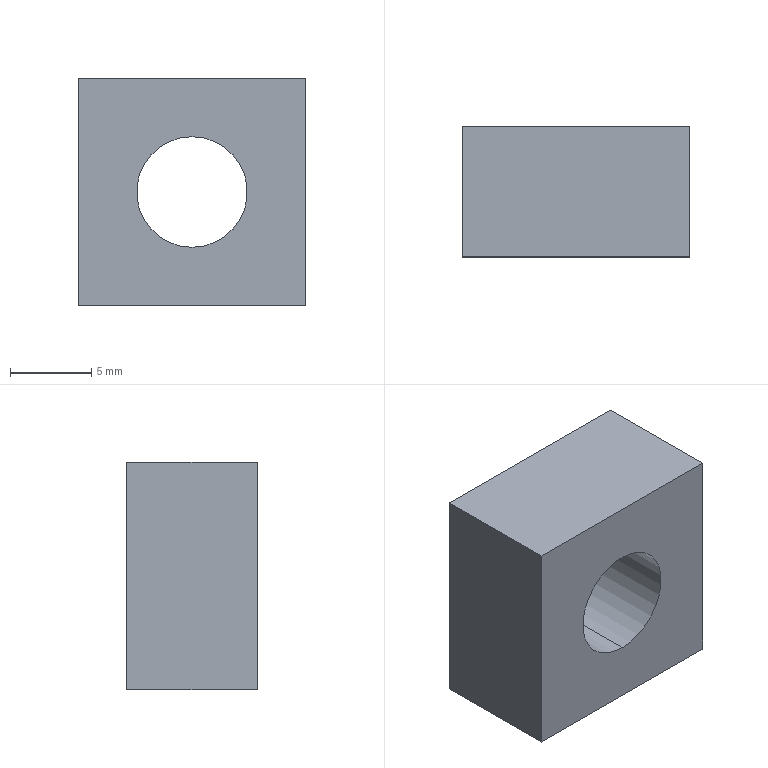Part | SolidWorks | features FlatPattern 1, HoleWzd 1, SMBaseFlange 1, SheetMetal 1 | 1 solid | 8 faces | box 14 x 8 x 14 mm | volume 1277 mm3 | plane 6 | cylinder 2 | commonest cylinder face diameters 6.8 x2
STEP:
#1=CARTESIAN_POINT('',(0.,0.,-3.4));
#2=VERTEX_POINT('',#1);
#3=CARTESIAN_POINT('',(0.,0.,3.4));
#4=VERTEX_POINT('',#3);
#5=CARTESIAN_POINT('',(0.,0.,0.));
#6=DIRECTION('',(0.,1.,0.));
#7=DIRECTION('',(0.,0.,1.));
#8=AXIS2_PLACEMENT_3D('',#5,#6,#7);
#9=CIRCLE('',#8,3.4);
#10=EDGE_CURVE('',#2,#4,#9,.T.);
#11=ORIENTED_EDGE('',*,*,#10,.F.);
#12=CARTESIAN_POINT('',(0.,8.,-3.4));
#13=VERTEX_POINT('',#12);
#14=CARTESIAN_POINT('',(0.,8.,-3.4));
#15=DIRECTION('',(0.,1.,0.));
#16=VECTOR('',#15,1000.);
#17=LINE('',#14,#16);
#18=EDGE_CURVE('',#2,#13,#17,.T.);
#19=ORIENTED_EDGE('',*,*,#18,.T.);
#20=CARTESIAN_POINT('',(0.,8.,3.4));
#21=VERTEX_POINT('',#20);
#22=CARTESIAN_POINT('',(0.,8.,0.));
#23=DIRECTION('',(0.,1.,0.));
#24=DIRECTION('',(0.,0.,1.));
#25=AXIS2_PLACEMENT_3D('',#22,#23,#24);
#26=CIRCLE('',#25,3.4);
#27=EDGE_CURVE('',#13,#21,#26,.T.);
#28=ORIENTED_EDGE('',*,*,#27,.T.);
#29=CARTESIAN_POINT('',(0.,8.,3.4));
#30=DIRECTION('',(0.,1.,0.));
#31=VECTOR('',#30,1000.);
#32=LINE('',#29,#31);
#33=EDGE_CURVE('',#4,#21,#32,.T.);
#34=ORIENTED_EDGE('',*,*,#33,.F.);
#35=EDGE_LOOP('',(#11,#19,#28,#34));
#36=FACE_OUTER_BOUND('',#35,.T.);
#37=CARTESIAN_POINT('',(0.,8.,0.));
#38=DIRECTION('',(0.,1.,0.));
#39=DIRECTION('',(0.,0.,1.));
#40=AXIS2_PLACEMENT_3D('',#37,#38,#39);
#41=CYLINDRICAL_SURFACE('',#40,3.4);
#42=ADVANCED_FACE('',(#36),#41,.F.);
#43=CARTESIAN_POINT('',(7.,0.,7.));
#44=VERTEX_POINT('',#43);
#45=CARTESIAN_POINT('',(7.,0.,-7.));
#46=VERTEX_POINT('',#45);
#47=CARTESIAN_POINT('',(7.,0.,-7.));
#48=DIRECTION('',(0.,0.,-1.));
#49=VECTOR('',#48,1000.);
#50=LINE('',#47,#49);
#51=EDGE_CURVE('',#44,#46,#50,.T.);
#52=ORIENTED_EDGE('',*,*,#51,.T.);
#53=CARTESIAN_POINT('',(7.,8.,-7.));
#54=VERTEX_POINT('',#53);
#55=CARTESIAN_POINT('',(7.,8.,-7.));
#56=DIRECTION('',(0.,-1.,0.));
#57=VECTOR('',#56,1000.);
#58=LINE('',#55,#57);
#59=EDGE_CURVE('',#54,#46,#58,.T.);
#60=ORIENTED_EDGE('',*,*,#59,.F.);
#61=CARTESIAN_POINT('',(7.,8.,7.));
#62=VERTEX_POINT('',#61);
#63=CARTESIAN_POINT('',(7.,8.,-7.));
#64=DIRECTION('',(0.,0.,-1.));
#65=VECTOR('',#64,1000.);
#66=LINE('',#63,#65);
#67=EDGE_CURVE('',#62,#54,#66,.T.);
#68=ORIENTED_EDGE('',*,*,#67,.F.);
#69=CARTESIAN_POINT('',(7.,8.,7.));
#70=DIRECTION('',(0.,-1.,0.));
#71=VECTOR('',#70,1000.);
#72=LINE('',#69,#71);
#73=EDGE_CURVE('',#62,#44,#72,.T.);
#74=ORIENTED_EDGE('',*,*,#73,.T.);
#75=EDGE_LOOP('',(#52,#60,#68,#74));
#76=FACE_OUTER_BOUND('',#75,.T.);
#77=CARTESIAN_POINT('',(7.,8.,-7.));
#78=DIRECTION('',(-1.,0.,0.));
#79=DIRECTION('',(0.,0.,1.));
#80=AXIS2_PLACEMENT_3D('',#77,#78,#79);
#81=PLANE('',#80);
#82=ADVANCED_FACE('',(#76),#81,.F.);
#83=CARTESIAN_POINT('',(-7.,0.,-7.));
#84=VERTEX_POINT('',#83);
#85=CARTESIAN_POINT('',(-7.,0.,-7.));
#86=DIRECTION('',(-1.,0.,0.));
#87=VECTOR('',#86,1000.);
#88=LINE('',#85,#87);
#89=EDGE_CURVE('',#46,#84,#88,.T.);
#90=ORIENTED_EDGE('',*,*,#89,.T.);
#91=CARTESIAN_POINT('',(-7.,8.,-7.));
#92=VERTEX_POINT('',#91);
#93=CARTESIAN_POINT('',(-7.,8.,-7.));
#94=DIRECTION('',(0.,-1.,0.));
#95=VECTOR('',#94,1000.);
#96=LINE('',#93,#95);
#97=EDGE_CURVE('',#92,#84,#96,.T.);
#98=ORIENTED_EDGE('',*,*,#97,.F.);
#99=CARTESIAN_POINT('',(-7.,8.,-7.));
#100=DIRECTION('',(-1.,0.,0.));
#101=VECTOR('',#100,1000.);
#102=LINE('',#99,#101);
#103=EDGE_CURVE('',#54,#92,#102,.T.);
#104=ORIENTED_EDGE('',*,*,#103,.F.);
#105=ORIENTED_EDGE('',*,*,#59,.T.);
#106=EDGE_LOOP('',(#90,#98,#104,#105));
#107=FACE_OUTER_BOUND('',#106,.T.);
#108=CARTESIAN_POINT('',(-7.,8.,-7.));
#109=DIRECTION('',(0.,0.,1.));
#110=DIRECTION('',(1.,0.,0.));
#111=AXIS2_PLACEMENT_3D('',#108,#109,#110);
#112=PLANE('',#111);
#113=ADVANCED_FACE('',(#107),#112,.F.);
#114=CARTESIAN_POINT('',(-7.,0.,7.));
#115=VERTEX_POINT('',#114);
#116=CARTESIAN_POINT('',(-7.,0.,-7.));
#117=DIRECTION('',(0.,0.,1.));
#118=VECTOR('',#117,1000.);
#119=LINE('',#116,#118);
#120=EDGE_CURVE('',#84,#115,#119,.T.);
#121=ORIENTED_EDGE('',*,*,#120,.T.);
#122=CARTESIAN_POINT('',(-7.,8.,7.));
#123=VERTEX_POINT('',#122);
#124=CARTESIAN_POINT('',(-7.,8.,7.));
#125=DIRECTION('',(0.,-1.,0.));
#126=VECTOR('',#125,1000.);
#127=LINE('',#124,#126);
#128=EDGE_CURVE('',#123,#115,#127,.T.);
#129=ORIENTED_EDGE('',*,*,#128,.F.);
#130=CARTESIAN_POINT('',(-7.,8.,-7.));
#131=DIRECTION('',(0.,0.,1.));
#132=VECTOR('',#131,1000.);
#133=LINE('',#130,#132);
#134=EDGE_CURVE('',#92,#123,#133,.T.);
#135=ORIENTED_EDGE('',*,*,#134,.F.);
#136=ORIENTED_EDGE('',*,*,#97,.T.);
#137=EDGE_LOOP('',(#121,#129,#135,#136));
#138=FACE_OUTER_BOUND('',#137,.T.);
#139=CARTESIAN_POINT('',(-7.,8.,-7.));
#140=DIRECTION('',(1.,0.,0.));
#141=DIRECTION('',(0.,0.,-1.));
#142=AXIS2_PLACEMENT_3D('',#139,#140,#141);
#143=PLANE('',#142);
#144=ADVANCED_FACE('',(#138),#143,.F.);
#145=CARTESIAN_POINT('',(-7.,0.,7.));
#146=DIRECTION('',(1.,0.,0.));
#147=VECTOR('',#146,1000.);
#148=LINE('',#145,#147);
#149=EDGE_CURVE('',#115,#44,#148,.T.);
#150=ORIENTED_EDGE('',*,*,#149,.T.);
#151=ORIENTED_EDGE('',*,*,#73,.F.);
#152=CARTESIAN_POINT('',(-7.,8.,7.));
#153=DIRECTION('',(1.,0.,0.));
#154=VECTOR('',#153,1000.);
#155=LINE('',#152,#154);
#156=EDGE_CURVE('',#123,#62,#155,.T.);
#157=ORIENTED_EDGE('',*,*,#156,.F.);
#158=ORIENTED_EDGE('',*,*,#128,.T.);
#159=EDGE_LOOP('',(#150,#151,#157,#158));
#160=FACE_OUTER_BOUND('',#159,.T.);
#161=CARTESIAN_POINT('',(-7.,8.,7.));
#162=DIRECTION('',(0.,0.,-1.));
#163=DIRECTION('',(-1.,0.,0.));
#164=AXIS2_PLACEMENT_3D('',#161,#162,#163);
#165=PLANE('',#164);
#166=ADVANCED_FACE('',(#160),#165,.F.);
#167=CARTESIAN_POINT('',(0.,8.,0.));
#168=DIRECTION('',(0.,1.,0.));
#169=DIRECTION('',(0.,0.,1.));
#170=AXIS2_PLACEMENT_3D('',#167,#168,#169);
#171=CIRCLE('',#170,3.4);
#172=EDGE_CURVE('',#21,#13,#171,.T.);
#173=ORIENTED_EDGE('',*,*,#172,.F.);
#174=ORIENTED_EDGE('',*,*,#27,.F.);
#175=EDGE_LOOP('',(#173,#174));
#176=FACE_BOUND('',#175,.T.);
#177=ORIENTED_EDGE('',*,*,#67,.T.);
#178=ORIENTED_EDGE('',*,*,#103,.T.);
#179=ORIENTED_EDGE('',*,*,#134,.T.);
#180=ORIENTED_EDGE('',*,*,#156,.T.);
#181=EDGE_LOOP('',(#177,#178,#179,#180));
#182=FACE_OUTER_BOUND('',#181,.T.);
#183=CARTESIAN_POINT('',(0.,8.,0.));
#184=DIRECTION('',(0.,1.,0.));
#185=DIRECTION('',(0.,0.,1.));
#186=AXIS2_PLACEMENT_3D('',#183,#184,#185);
#187=PLANE('',#186);
#188=ADVANCED_FACE('',(#176,#182),#187,.T.);
#189=CARTESIAN_POINT('',(0.,0.,0.));
#190=DIRECTION('',(0.,1.,0.));
#191=DIRECTION('',(0.,0.,1.));
#192=AXIS2_PLACEMENT_3D('',#189,#190,#191);
#193=CIRCLE('',#192,3.4);
#194=EDGE_CURVE('',#4,#2,#193,.T.);
#195=ORIENTED_EDGE('',*,*,#194,.T.);
#196=ORIENTED_EDGE('',*,*,#10,.T.);
#197=EDGE_LOOP('',(#195,#196));
#198=FACE_BOUND('',#197,.T.);
#199=ORIENTED_EDGE('',*,*,#51,.F.);
#200=ORIENTED_EDGE('',*,*,#149,.F.);
#201=ORIENTED_EDGE('',*,*,#120,.F.);
#202=ORIENTED_EDGE('',*,*,#89,.F.);
#203=EDGE_LOOP('',(#199,#200,#201,#202));
#204=FACE_OUTER_BOUND('',#203,.T.);
#205=CARTESIAN_POINT('',(0.,0.,0.));
#206=DIRECTION('',(0.,1.,0.));
#207=DIRECTION('',(0.,0.,1.));
#208=AXIS2_PLACEMENT_3D('',#205,#206,#207);
#209=PLANE('',#208);
#210=ADVANCED_FACE('',(#198,#204),#209,.F.);
#211=ORIENTED_EDGE('',*,*,#18,.F.);
#212=ORIENTED_EDGE('',*,*,#194,.F.);
#213=ORIENTED_EDGE('',*,*,#33,.T.);
#214=ORIENTED_EDGE('',*,*,#172,.T.);
#215=EDGE_LOOP('',(#211,#212,#213,#214));
#216=FACE_OUTER_BOUND('',#215,.T.);
#217=CARTESIAN_POINT('',(0.,8.,0.));
#218=DIRECTION('',(0.,1.,0.));
#219=DIRECTION('',(0.,0.,1.));
#220=AXIS2_PLACEMENT_3D('',#217,#218,#219);
#221=CYLINDRICAL_SURFACE('',#220,3.4);
#222=ADVANCED_FACE('',(#216),#221,.F.);
#223=CLOSED_SHELL('',(#42,#82,#113,#144,#166,#188,#210,#222));
#224=MANIFOLD_SOLID_BREP('',#223);
#225=CARTESIAN_POINT('',(0.,0.,0.));
#226=DIRECTION('',(0.,0.,1.));
#227=DIRECTION('',(1.,0.,0.));
#228=AXIS2_PLACEMENT_3D('',#225,#226,#227);
#229=(LENGTH_UNIT()NAMED_UNIT(*)SI_UNIT(.MILLI.,.METRE.));
#230=UNCERTAINTY_MEASURE_WITH_UNIT(LENGTH_MEASURE(0.00001),#229,'','');
#231=(NAMED_UNIT(*)PLANE_ANGLE_UNIT()SI_UNIT($,.RADIAN.));
#232=(NAMED_UNIT(*)SI_UNIT($,.STERADIAN.)SOLID_ANGLE_UNIT());
#233=(GEOMETRIC_REPRESENTATION_CONTEXT(3)GLOBAL_UNCERTAINTY_ASSIGNED_CONTEXT((#230))GLOBAL_UNIT_ASSIGNED_CONTEXT((#229,#231,#232))REPRESENTATION_CONTEXT('',''));
#234=ADVANCED_BREP_SHAPE_REPRESENTATION('',(#224,#228),#233);